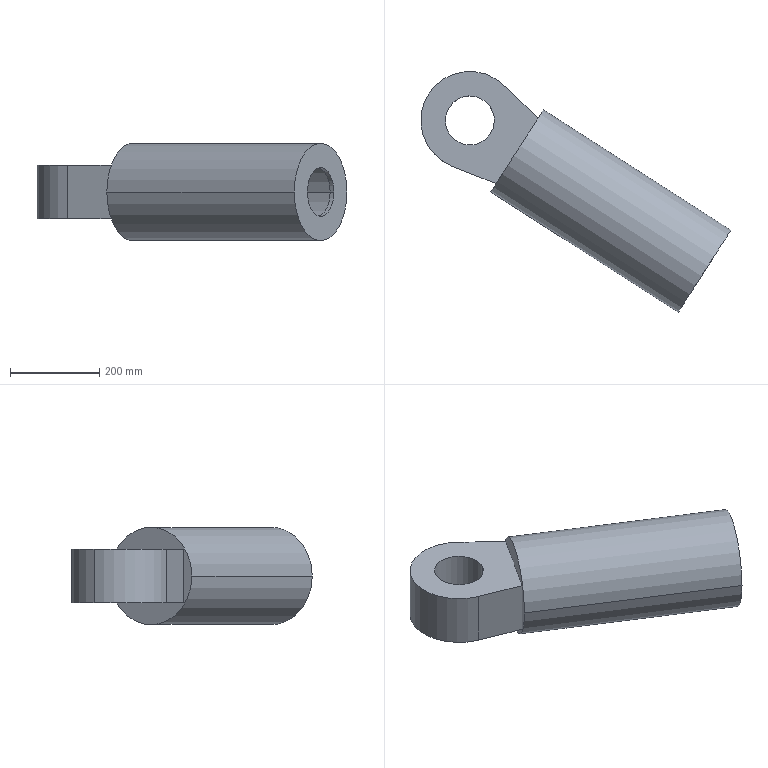Part | SolidWorks | features SplitBody 1 | 1 solid | 18 faces | box 696.192 x 540.383 x 219 mm | volume 10939320 mm3 | cylinder 10 | plane 8 | commonest cylinder face diameters 110 x4 180 x2 219 x2 220 x2
STEP:
#1=CARTESIAN_POINT('',(4022.192,522.369,927.5));
#2=VERTEX_POINT('',#1);
#3=CARTESIAN_POINT('',(3903.913,338.057,927.5));
#4=VERTEX_POINT('',#3);
#5=CARTESIAN_POINT('',(3963.053,430.213,927.5));
#6=DIRECTION('',(-0.8416,0.5401,0.));
#7=DIRECTION('',(0.5401,0.8416,0.));
#8=AXIS2_PLACEMENT_3D('',#5,#6,#7);
#9=CIRCLE('',#8,109.5);
#10=EDGE_CURVE('',#2,#4,#9,.T.);
#11=ORIENTED_EDGE('',*,*,#10,.T.);
#12=CARTESIAN_POINT('',(3483.109,608.101,927.5));
#13=VERTEX_POINT('',#12);
#14=CARTESIAN_POINT('',(3903.913,338.057,927.5));
#15=DIRECTION('',(-0.8416,0.5401,0.));
#16=VECTOR('',#15,1000.);
#17=LINE('',#14,#16);
#18=EDGE_CURVE('',#4,#13,#17,.T.);
#19=ORIENTED_EDGE('',*,*,#18,.T.);
#20=CARTESIAN_POINT('',(3601.388,792.413,927.5));
#21=VERTEX_POINT('',#20);
#22=CARTESIAN_POINT('',(3542.248,700.257,927.5));
#23=DIRECTION('',(0.8416,-0.5401,0.));
#24=DIRECTION('',(0.5401,0.8416,0.));
#25=AXIS2_PLACEMENT_3D('',#22,#23,#24);
#26=CIRCLE('',#25,109.5);
#27=EDGE_CURVE('',#13,#21,#26,.T.);
#28=ORIENTED_EDGE('',*,*,#27,.T.);
#29=CARTESIAN_POINT('',(4022.192,522.369,927.5));
#30=DIRECTION('',(-0.8416,0.5401,0.));
#31=VECTOR('',#30,1000.);
#32=LINE('',#29,#31);
#33=EDGE_CURVE('',#2,#21,#32,.T.);
#34=ORIENTED_EDGE('',*,*,#33,.F.);
#35=EDGE_LOOP('',(#11,#19,#28,#34));
#36=FACE_OUTER_BOUND('',#35,.T.);
#37=CARTESIAN_POINT('',(3963.053,430.213,927.5));
#38=DIRECTION('',(-0.8416,0.5401,0.));
#39=DIRECTION('',(0.5401,0.8416,0.));
#40=AXIS2_PLACEMENT_3D('',#37,#38,#39);
#41=CYLINDRICAL_SURFACE('',#40,109.5);
#42=ADVANCED_FACE('',(#36),#41,.T.);
#43=CARTESIAN_POINT('',(3984.341,481.902,927.5));
#44=VERTEX_POINT('',#43);
#45=CARTESIAN_POINT('',(3924.932,389.325,927.5));
#46=VERTEX_POINT('',#45);
#47=CARTESIAN_POINT('',(3954.637,435.614,927.5));
#48=DIRECTION('',(0.8416,-0.5401,0.));
#49=DIRECTION('',(-0.5401,-0.8416,0.));
#50=AXIS2_PLACEMENT_3D('',#47,#48,#49);
#51=CIRCLE('',#50,55.);
#52=EDGE_CURVE('',#44,#46,#51,.T.);
#53=ORIENTED_EDGE('',*,*,#52,.F.);
#54=CARTESIAN_POINT('',(3992.757,476.501,927.5));
#55=VERTEX_POINT('',#54);
#56=CARTESIAN_POINT('',(3984.341,481.902,927.5));
#57=DIRECTION('',(0.8416,-0.5401,0.));
#58=VECTOR('',#57,1000.);
#59=LINE('',#56,#58);
#60=EDGE_CURVE('',#44,#55,#59,.T.);
#61=ORIENTED_EDGE('',*,*,#60,.T.);
#62=CARTESIAN_POINT('',(3933.348,383.924,927.5));
#63=VERTEX_POINT('',#62);
#64=CARTESIAN_POINT('',(3963.053,430.213,927.5));
#65=DIRECTION('',(-0.8416,0.5401,0.));
#66=DIRECTION('',(-0.5401,-0.8416,0.));
#67=AXIS2_PLACEMENT_3D('',#64,#65,#66);
#68=CIRCLE('',#67,55.);
#69=EDGE_CURVE('',#63,#55,#68,.T.);
#70=ORIENTED_EDGE('',*,*,#69,.F.);
#71=CARTESIAN_POINT('',(3924.932,389.325,927.5));
#72=DIRECTION('',(0.8416,-0.5401,0.));
#73=VECTOR('',#72,1000.);
#74=LINE('',#71,#73);
#75=EDGE_CURVE('',#46,#63,#74,.T.);
#76=ORIENTED_EDGE('',*,*,#75,.F.);
#77=EDGE_LOOP('',(#53,#61,#70,#76));
#78=FACE_OUTER_BOUND('',#77,.T.);
#79=CARTESIAN_POINT('',(3954.637,435.614,927.5));
#80=DIRECTION('',(0.8416,-0.5401,0.));
#81=DIRECTION('',(-0.5401,-0.8416,0.));
#82=AXIS2_PLACEMENT_3D('',#79,#80,#81);
#83=CYLINDRICAL_SURFACE('',#82,55.);
#84=ADVANCED_FACE('',(#78),#83,.F.);
#85=CARTESIAN_POINT('',(3343.423,827.85,867.5));
#86=VERTEX_POINT('',#85);
#87=CARTESIAN_POINT('',(3511.997,847.967,867.5));
#88=VERTEX_POINT('',#87);
#89=CARTESIAN_POINT('',(3436.,768.44,867.5));
#90=DIRECTION('',(0.,0.,-1.));
#91=DIRECTION('',(-0.8416,0.5401,0.));
#92=AXIS2_PLACEMENT_3D('',#89,#90,#91);
#93=CIRCLE('',#92,110.);
#94=EDGE_CURVE('',#86,#88,#93,.T.);
#95=ORIENTED_EDGE('',*,*,#94,.F.);
#96=CARTESIAN_POINT('',(3343.423,827.85,987.5));
#97=VERTEX_POINT('',#96);
#98=CARTESIAN_POINT('',(3343.423,827.85,867.5));
#99=DIRECTION('',(0.,0.,1.));
#100=VECTOR('',#99,1000.);
#101=LINE('',#98,#100);
#102=EDGE_CURVE('',#86,#97,#101,.T.);
#103=ORIENTED_EDGE('',*,*,#102,.T.);
#104=CARTESIAN_POINT('',(3511.997,847.967,987.5));
#105=VERTEX_POINT('',#104);
#106=CARTESIAN_POINT('',(3436.,768.44,987.5));
#107=DIRECTION('',(0.,0.,-1.));
#108=DIRECTION('',(-0.8416,0.5401,0.));
#109=AXIS2_PLACEMENT_3D('',#106,#107,#108);
#110=CIRCLE('',#109,110.);
#111=EDGE_CURVE('',#97,#105,#110,.T.);
#112=ORIENTED_EDGE('',*,*,#111,.T.);
#113=CARTESIAN_POINT('',(3511.997,847.967,867.5));
#114=DIRECTION('',(0.,0.,-1.));
#115=VECTOR('',#114,1000.);
#116=LINE('',#113,#115);
#117=EDGE_CURVE('',#105,#88,#116,.T.);
#118=ORIENTED_EDGE('',*,*,#117,.T.);
#119=EDGE_LOOP('',(#95,#103,#112,#118));
#120=FACE_OUTER_BOUND('',#119,.T.);
#121=CARTESIAN_POINT('',(3436.,768.44,867.5));
#122=DIRECTION('',(0.,0.,1.));
#123=DIRECTION('',(-0.8416,0.5401,0.));
#124=AXIS2_PLACEMENT_3D('',#121,#122,#123);
#125=CYLINDRICAL_SURFACE('',#124,110.);
#126=ADVANCED_FACE('',(#120),#125,.T.);
#127=CARTESIAN_POINT('',(3482.288,738.735,867.5));
#128=VERTEX_POINT('',#127);
#129=CARTESIAN_POINT('',(3389.712,798.145,867.5));
#130=VERTEX_POINT('',#129);
#131=CARTESIAN_POINT('',(3436.,768.44,867.5));
#132=DIRECTION('',(0.,0.,1.));
#133=DIRECTION('',(-0.8416,0.5401,0.));
#134=AXIS2_PLACEMENT_3D('',#131,#132,#133);
#135=CIRCLE('',#134,55.);
#136=EDGE_CURVE('',#128,#130,#135,.T.);
#137=ORIENTED_EDGE('',*,*,#136,.F.);
#138=CARTESIAN_POINT('',(3482.288,738.735,987.5));
#139=VERTEX_POINT('',#138);
#140=CARTESIAN_POINT('',(3482.288,738.735,867.5));
#141=DIRECTION('',(0.,0.,1.));
#142=VECTOR('',#141,1000.);
#143=LINE('',#140,#142);
#144=EDGE_CURVE('',#128,#139,#143,.T.);
#145=ORIENTED_EDGE('',*,*,#144,.T.);
#146=CARTESIAN_POINT('',(3389.712,798.145,987.5));
#147=VERTEX_POINT('',#146);
#148=CARTESIAN_POINT('',(3436.,768.44,987.5));
#149=DIRECTION('',(0.,0.,1.));
#150=DIRECTION('',(-0.8416,0.5401,0.));
#151=AXIS2_PLACEMENT_3D('',#148,#149,#150);
#152=CIRCLE('',#151,55.);
#153=EDGE_CURVE('',#139,#147,#152,.T.);
#154=ORIENTED_EDGE('',*,*,#153,.T.);
#155=CARTESIAN_POINT('',(3389.712,798.145,867.5));
#156=DIRECTION('',(0.,0.,1.));
#157=VECTOR('',#156,1000.);
#158=LINE('',#155,#157);
#159=EDGE_CURVE('',#130,#147,#158,.T.);
#160=ORIENTED_EDGE('',*,*,#159,.F.);
#161=EDGE_LOOP('',(#137,#145,#154,#160));
#162=FACE_OUTER_BOUND('',#161,.T.);
#163=CARTESIAN_POINT('',(3436.,768.44,867.5));
#164=DIRECTION('',(0.,0.,1.));
#165=DIRECTION('',(-0.8416,0.5401,0.));
#166=AXIS2_PLACEMENT_3D('',#163,#164,#165);
#167=CYLINDRICAL_SURFACE('',#166,55.);
#168=ADVANCED_FACE('',(#162),#167,.F.);
#169=CARTESIAN_POINT('',(3607.689,765.2,927.5));
#170=VERTEX_POINT('',#169);
#171=CARTESIAN_POINT('',(3510.473,613.71,927.5));
#172=VERTEX_POINT('',#171);
#173=CARTESIAN_POINT('',(3559.081,689.455,927.5));
#174=DIRECTION('',(0.8416,-0.5401,0.));
#175=DIRECTION('',(-0.5401,-0.8416,0.));
#176=AXIS2_PLACEMENT_3D('',#173,#174,#175);
#177=CIRCLE('',#176,90.);
#178=EDGE_CURVE('',#170,#172,#177,.T.);
#179=ORIENTED_EDGE('',*,*,#178,.F.);
#180=CARTESIAN_POINT('',(4003.244,511.358,927.5));
#181=VERTEX_POINT('',#180);
#182=CARTESIAN_POINT('',(3607.689,765.2,927.5));
#183=DIRECTION('',(0.8416,-0.5401,0.));
#184=VECTOR('',#183,1000.);
#185=LINE('',#182,#184);
#186=EDGE_CURVE('',#170,#181,#185,.T.);
#187=ORIENTED_EDGE('',*,*,#186,.T.);
#188=CARTESIAN_POINT('',(3906.029,359.869,927.5));
#189=VERTEX_POINT('',#188);
#190=CARTESIAN_POINT('',(3954.637,435.614,927.5));
#191=DIRECTION('',(0.8416,-0.5401,0.));
#192=DIRECTION('',(-0.5401,-0.8416,0.));
#193=AXIS2_PLACEMENT_3D('',#190,#191,#192);
#194=CIRCLE('',#193,90.);
#195=EDGE_CURVE('',#181,#189,#194,.T.);
#196=ORIENTED_EDGE('',*,*,#195,.T.);
#197=CARTESIAN_POINT('',(3510.473,613.71,927.5));
#198=DIRECTION('',(0.8416,-0.5401,0.));
#199=VECTOR('',#198,1000.);
#200=LINE('',#197,#199);
#201=EDGE_CURVE('',#172,#189,#200,.T.);
#202=ORIENTED_EDGE('',*,*,#201,.F.);
#203=EDGE_LOOP('',(#179,#187,#196,#202));
#204=FACE_OUTER_BOUND('',#203,.T.);
#205=CARTESIAN_POINT('',(3559.081,689.455,927.5));
#206=DIRECTION('',(0.8416,-0.5401,0.));
#207=DIRECTION('',(-0.5401,-0.8416,0.));
#208=AXIS2_PLACEMENT_3D('',#205,#206,#207);
#209=CYLINDRICAL_SURFACE('',#208,90.);
#210=ADVANCED_FACE('',(#204),#209,.F.);
#211=ORIENTED_EDGE('',*,*,#18,.F.);
#212=CARTESIAN_POINT('',(3963.053,430.213,927.5));
#213=DIRECTION('',(-0.8416,0.5401,0.));
#214=DIRECTION('',(0.5401,0.8416,0.));
#215=AXIS2_PLACEMENT_3D('',#212,#213,#214);
#216=CIRCLE('',#215,109.5);
#217=EDGE_CURVE('',#4,#2,#216,.T.);
#218=ORIENTED_EDGE('',*,*,#217,.T.);
#219=ORIENTED_EDGE('',*,*,#33,.T.);
#220=CARTESIAN_POINT('',(3542.248,700.257,927.5));
#221=DIRECTION('',(0.8416,-0.5401,0.));
#222=DIRECTION('',(0.5401,0.8416,0.));
#223=AXIS2_PLACEMENT_3D('',#220,#221,#222);
#224=CIRCLE('',#223,109.5);
#225=EDGE_CURVE('',#21,#13,#224,.T.);
#226=ORIENTED_EDGE('',*,*,#225,.T.);
#227=EDGE_LOOP('',(#211,#218,#219,#226));
#228=FACE_OUTER_BOUND('',#227,.T.);
#229=CARTESIAN_POINT('',(3963.053,430.213,927.5));
#230=DIRECTION('',(-0.8416,0.5401,0.));
#231=DIRECTION('',(0.5401,0.8416,0.));
#232=AXIS2_PLACEMENT_3D('',#229,#230,#231);
#233=CYLINDRICAL_SURFACE('',#232,109.5);
#234=ADVANCED_FACE('',(#228),#233,.T.);
#235=CARTESIAN_POINT('',(3494.991,626.616,987.5));
#236=VERTEX_POINT('',#235);
#237=CARTESIAN_POINT('',(3589.506,773.898,987.5));
#238=VERTEX_POINT('',#237);
#239=CARTESIAN_POINT('',(3542.248,700.257,987.5));
#240=DIRECTION('',(0.5401,0.8416,0.));
#241=VECTOR('',#240,1000.);
#242=LINE('',#239,#241);
#243=EDGE_CURVE('',#236,#238,#242,.T.);
#244=ORIENTED_EDGE('',*,*,#243,.F.);
#245=CARTESIAN_POINT('',(3494.991,626.616,867.5));
#246=VERTEX_POINT('',#245);
#247=CARTESIAN_POINT('',(3494.991,626.616,927.5));
#248=DIRECTION('',(0.,0.,1.));
#249=VECTOR('',#248,1000.);
#250=LINE('',#247,#249);
#251=EDGE_CURVE('',#246,#236,#250,.T.);
#252=ORIENTED_EDGE('',*,*,#251,.F.);
#253=CARTESIAN_POINT('',(3589.506,773.898,867.5));
#254=VERTEX_POINT('',#253);
#255=CARTESIAN_POINT('',(3542.248,700.257,867.5));
#256=DIRECTION('',(-0.5401,-0.8416,0.));
#257=VECTOR('',#256,1000.);
#258=LINE('',#255,#257);
#259=EDGE_CURVE('',#254,#246,#258,.T.);
#260=ORIENTED_EDGE('',*,*,#259,.F.);
#261=CARTESIAN_POINT('',(3589.506,773.898,927.5));
#262=DIRECTION('',(0.,0.,-1.));
#263=VECTOR('',#262,1000.);
#264=LINE('',#261,#263);
#265=EDGE_CURVE('',#238,#254,#264,.T.);
#266=ORIENTED_EDGE('',*,*,#265,.F.);
#267=EDGE_LOOP('',(#244,#252,#260,#266));
#268=FACE_BOUND('',#267,.T.);
#269=ORIENTED_EDGE('',*,*,#225,.F.);
#270=ORIENTED_EDGE('',*,*,#27,.F.);
#271=EDGE_LOOP('',(#269,#270));
#272=FACE_OUTER_BOUND('',#271,.T.);
#273=CARTESIAN_POINT('',(3542.248,700.257,927.5));
#274=DIRECTION('',(0.8416,-0.5401,0.));
#275=DIRECTION('',(-0.5401,-0.8416,0.));
#276=AXIS2_PLACEMENT_3D('',#273,#274,#275);
#277=PLANE('',#276);
#278=ADVANCED_FACE('',(#268,#272),#277,.F.);
#279=ORIENTED_EDGE('',*,*,#69,.T.);
#280=CARTESIAN_POINT('',(3963.053,430.213,927.5));
#281=DIRECTION('',(-0.8416,0.5401,0.));
#282=DIRECTION('',(-0.5401,-0.8416,0.));
#283=AXIS2_PLACEMENT_3D('',#280,#281,#282);
#284=CIRCLE('',#283,55.);
#285=EDGE_CURVE('',#55,#63,#284,.T.);
#286=ORIENTED_EDGE('',*,*,#285,.T.);
#287=EDGE_LOOP('',(#279,#286));
#288=FACE_BOUND('',#287,.T.);
#289=ORIENTED_EDGE('',*,*,#10,.F.);
#290=ORIENTED_EDGE('',*,*,#217,.F.);
#291=EDGE_LOOP('',(#289,#290));
#292=FACE_OUTER_BOUND('',#291,.T.);
#293=CARTESIAN_POINT('',(3963.053,430.213,927.5));
#294=DIRECTION('',(0.8416,-0.5401,0.));
#295=DIRECTION('',(-0.5401,-0.8416,0.));
#296=AXIS2_PLACEMENT_3D('',#293,#294,#295);
#297=PLANE('',#296);
#298=ADVANCED_FACE('',(#288,#292),#297,.T.);
#299=ORIENTED_EDGE('',*,*,#265,.T.);
#300=CARTESIAN_POINT('',(3511.997,847.967,867.5));
#301=DIRECTION('',(0.723,-0.6909,0.));
#302=VECTOR('',#301,1000.);
#303=LINE('',#300,#302);
#304=EDGE_CURVE('',#88,#254,#303,.T.);
#305=ORIENTED_EDGE('',*,*,#304,.F.);
#306=ORIENTED_EDGE('',*,*,#117,.F.);
#307=CARTESIAN_POINT('',(3511.997,847.967,987.5));
#308=DIRECTION('',(-0.723,0.6909,0.));
#309=VECTOR('',#308,1000.);
#310=LINE('',#307,#309);
#311=EDGE_CURVE('',#238,#105,#310,.T.);
#312=ORIENTED_EDGE('',*,*,#311,.F.);
#313=EDGE_LOOP('',(#299,#305,#306,#312));
#314=FACE_OUTER_BOUND('',#313,.T.);
#315=CARTESIAN_POINT('',(3511.997,847.967,867.5));
#316=DIRECTION('',(-0.6909,-0.723,0.));
#317=DIRECTION('',(-0.723,0.6909,0.));
#318=AXIS2_PLACEMENT_3D('',#315,#316,#317);
#319=PLANE('',#318);
#320=ADVANCED_FACE('',(#314),#319,.F.);
#321=CARTESIAN_POINT('',(3436.,768.44,987.5));
#322=DIRECTION('',(0.,0.,1.));
#323=DIRECTION('',(-0.8416,0.5401,0.));
#324=AXIS2_PLACEMENT_3D('',#321,#322,#323);
#325=CIRCLE('',#324,55.);
#326=EDGE_CURVE('',#147,#139,#325,.T.);
#327=ORIENTED_EDGE('',*,*,#326,.F.);
#328=ORIENTED_EDGE('',*,*,#153,.F.);
#329=EDGE_LOOP('',(#327,#328));
#330=FACE_BOUND('',#329,.T.);
#331=CARTESIAN_POINT('',(3395.364,666.221,987.5));
#332=VERTEX_POINT('',#331);
#333=CARTESIAN_POINT('',(3494.991,626.616,987.5));
#334=DIRECTION('',(-0.9293,0.3694,0.));
#335=VECTOR('',#334,1000.);
#336=LINE('',#333,#335);
#337=EDGE_CURVE('',#236,#332,#336,.T.);
#338=ORIENTED_EDGE('',*,*,#337,.F.);
#339=ORIENTED_EDGE('',*,*,#243,.T.);
#340=ORIENTED_EDGE('',*,*,#311,.T.);
#341=ORIENTED_EDGE('',*,*,#111,.F.);
#342=CARTESIAN_POINT('',(3436.,768.44,987.5));
#343=DIRECTION('',(0.,0.,-1.));
#344=DIRECTION('',(-0.8416,0.5401,0.));
#345=AXIS2_PLACEMENT_3D('',#342,#343,#344);
#346=CIRCLE('',#345,110.);
#347=EDGE_CURVE('',#332,#97,#346,.T.);
#348=ORIENTED_EDGE('',*,*,#347,.F.);
#349=EDGE_LOOP('',(#338,#339,#340,#341,#348));
#350=FACE_OUTER_BOUND('',#349,.T.);
#351=CARTESIAN_POINT('',(3436.,768.44,987.5));
#352=DIRECTION('',(0.,0.,-1.));
#353=DIRECTION('',(0.8416,-0.5401,0.));
#354=AXIS2_PLACEMENT_3D('',#351,#352,#353);
#355=PLANE('',#354);
#356=ADVANCED_FACE('',(#330,#350),#355,.F.);
#357=CARTESIAN_POINT('',(3395.364,666.221,867.5));
#358=VERTEX_POINT('',#357);
#359=CARTESIAN_POINT('',(3395.364,666.221,867.5));
#360=DIRECTION('',(0.,0.,1.));
#361=VECTOR('',#360,1000.);
#362=LINE('',#359,#361);
#363=EDGE_CURVE('',#358,#332,#362,.T.);
#364=ORIENTED_EDGE('',*,*,#363,.F.);
#365=CARTESIAN_POINT('',(3395.364,666.221,867.5));
#366=DIRECTION('',(-0.9293,0.3694,0.));
#367=VECTOR('',#366,1000.);
#368=LINE('',#365,#367);
#369=EDGE_CURVE('',#246,#358,#368,.T.);
#370=ORIENTED_EDGE('',*,*,#369,.F.);
#371=ORIENTED_EDGE('',*,*,#251,.T.);
#372=ORIENTED_EDGE('',*,*,#337,.T.);
#373=EDGE_LOOP('',(#364,#370,#371,#372));
#374=FACE_OUTER_BOUND('',#373,.T.);
#375=CARTESIAN_POINT('',(3395.364,666.221,867.5));
#376=DIRECTION('',(0.3694,0.9293,0.));
#377=DIRECTION('',(0.9293,-0.3694,0.));
#378=AXIS2_PLACEMENT_3D('',#375,#376,#377);
#379=PLANE('',#378);
#380=ADVANCED_FACE('',(#374),#379,.F.);
#381=CARTESIAN_POINT('',(3436.,768.44,867.5));
#382=DIRECTION('',(0.,0.,1.));
#383=DIRECTION('',(-0.8416,0.5401,0.));
#384=AXIS2_PLACEMENT_3D('',#381,#382,#383);
#385=CIRCLE('',#384,55.);
#386=EDGE_CURVE('',#130,#128,#385,.T.);
#387=ORIENTED_EDGE('',*,*,#386,.T.);
#388=ORIENTED_EDGE('',*,*,#136,.T.);
#389=EDGE_LOOP('',(#387,#388));
#390=FACE_BOUND('',#389,.T.);
#391=ORIENTED_EDGE('',*,*,#259,.T.);
#392=ORIENTED_EDGE('',*,*,#369,.T.);
#393=CARTESIAN_POINT('',(3436.,768.44,867.5));
#394=DIRECTION('',(0.,0.,-1.));
#395=DIRECTION('',(-0.8416,0.5401,0.));
#396=AXIS2_PLACEMENT_3D('',#393,#394,#395);
#397=CIRCLE('',#396,110.);
#398=EDGE_CURVE('',#358,#86,#397,.T.);
#399=ORIENTED_EDGE('',*,*,#398,.T.);
#400=ORIENTED_EDGE('',*,*,#94,.T.);
#401=ORIENTED_EDGE('',*,*,#304,.T.);
#402=EDGE_LOOP('',(#391,#392,#399,#400,#401));
#403=FACE_OUTER_BOUND('',#402,.T.);
#404=CARTESIAN_POINT('',(3436.,768.44,867.5));
#405=DIRECTION('',(0.,0.,-1.));
#406=DIRECTION('',(0.8416,-0.5401,0.));
#407=AXIS2_PLACEMENT_3D('',#404,#405,#406);
#408=PLANE('',#407);
#409=ADVANCED_FACE('',(#390,#403),#408,.T.);
#410=ORIENTED_EDGE('',*,*,#60,.F.);
#411=CARTESIAN_POINT('',(3954.637,435.614,927.5));
#412=DIRECTION('',(0.8416,-0.5401,0.));
#413=DIRECTION('',(-0.5401,-0.8416,0.));
#414=AXIS2_PLACEMENT_3D('',#411,#412,#413);
#415=CIRCLE('',#414,55.);
#416=EDGE_CURVE('',#46,#44,#415,.T.);
#417=ORIENTED_EDGE('',*,*,#416,.F.);
#418=ORIENTED_EDGE('',*,*,#75,.T.);
#419=ORIENTED_EDGE('',*,*,#285,.F.);
#420=EDGE_LOOP('',(#410,#417,#418,#419));
#421=FACE_OUTER_BOUND('',#420,.T.);
#422=CARTESIAN_POINT('',(3954.637,435.614,927.5));
#423=DIRECTION('',(0.8416,-0.5401,0.));
#424=DIRECTION('',(-0.5401,-0.8416,0.));
#425=AXIS2_PLACEMENT_3D('',#422,#423,#424);
#426=CYLINDRICAL_SURFACE('',#425,55.);
#427=ADVANCED_FACE('',(#421),#426,.F.);
#428=ORIENTED_EDGE('',*,*,#102,.F.);
#429=ORIENTED_EDGE('',*,*,#398,.F.);
#430=ORIENTED_EDGE('',*,*,#363,.T.);
#431=ORIENTED_EDGE('',*,*,#347,.T.);
#432=EDGE_LOOP('',(#428,#429,#430,#431));
#433=FACE_OUTER_BOUND('',#432,.T.);
#434=CARTESIAN_POINT('',(3436.,768.44,867.5));
#435=DIRECTION('',(0.,0.,1.));
#436=DIRECTION('',(-0.8416,0.5401,0.));
#437=AXIS2_PLACEMENT_3D('',#434,#435,#436);
#438=CYLINDRICAL_SURFACE('',#437,110.);
#439=ADVANCED_FACE('',(#433),#438,.T.);
#440=ORIENTED_EDGE('',*,*,#144,.F.);
#441=ORIENTED_EDGE('',*,*,#386,.F.);
#442=ORIENTED_EDGE('',*,*,#159,.T.);
#443=ORIENTED_EDGE('',*,*,#326,.T.);
#444=EDGE_LOOP('',(#440,#441,#442,#443));
#445=FACE_OUTER_BOUND('',#444,.T.);
#446=CARTESIAN_POINT('',(3436.,768.44,867.5));
#447=DIRECTION('',(0.,0.,1.));
#448=DIRECTION('',(-0.8416,0.5401,0.));
#449=AXIS2_PLACEMENT_3D('',#446,#447,#448);
#450=CYLINDRICAL_SURFACE('',#449,55.);
#451=ADVANCED_FACE('',(#445),#450,.F.);
#452=CARTESIAN_POINT('',(3954.637,435.614,927.5));
#453=DIRECTION('',(0.8416,-0.5401,0.));
#454=DIRECTION('',(-0.5401,-0.8416,0.));
#455=AXIS2_PLACEMENT_3D('',#452,#453,#454);
#456=CIRCLE('',#455,90.);
#457=EDGE_CURVE('',#189,#181,#456,.T.);
#458=ORIENTED_EDGE('',*,*,#457,.F.);
#459=ORIENTED_EDGE('',*,*,#195,.F.);
#460=EDGE_LOOP('',(#458,#459));
#461=FACE_OUTER_BOUND('',#460,.T.);
#462=ORIENTED_EDGE('',*,*,#416,.T.);
#463=ORIENTED_EDGE('',*,*,#52,.T.);
#464=EDGE_LOOP('',(#462,#463));
#465=FACE_BOUND('',#464,.T.);
#466=CARTESIAN_POINT('',(3954.637,435.614,927.5));
#467=DIRECTION('',(0.8416,-0.5401,0.));
#468=DIRECTION('',(-0.5401,-0.8416,0.));
#469=AXIS2_PLACEMENT_3D('',#466,#467,#468);
#470=PLANE('',#469);
#471=ADVANCED_FACE('',(#461,#465),#470,.F.);
#472=ORIENTED_EDGE('',*,*,#186,.F.);
#473=CARTESIAN_POINT('',(3559.081,689.455,927.5));
#474=DIRECTION('',(0.8416,-0.5401,0.));
#475=DIRECTION('',(-0.5401,-0.8416,0.));
#476=AXIS2_PLACEMENT_3D('',#473,#474,#475);
#477=CIRCLE('',#476,90.);
#478=EDGE_CURVE('',#172,#170,#477,.T.);
#479=ORIENTED_EDGE('',*,*,#478,.F.);
#480=ORIENTED_EDGE('',*,*,#201,.T.);
#481=ORIENTED_EDGE('',*,*,#457,.T.);
#482=EDGE_LOOP('',(#472,#479,#480,#481));
#483=FACE_OUTER_BOUND('',#482,.T.);
#484=CARTESIAN_POINT('',(3559.081,689.455,927.5));
#485=DIRECTION('',(0.8416,-0.5401,0.));
#486=DIRECTION('',(-0.5401,-0.8416,0.));
#487=AXIS2_PLACEMENT_3D('',#484,#485,#486);
#488=CYLINDRICAL_SURFACE('',#487,90.);
#489=ADVANCED_FACE('',(#483),#488,.F.);
#490=ORIENTED_EDGE('',*,*,#478,.T.);
#491=ORIENTED_EDGE('',*,*,#178,.T.);
#492=EDGE_LOOP('',(#490,#491));
#493=FACE_OUTER_BOUND('',#492,.T.);
#494=CARTESIAN_POINT('',(3559.081,689.455,927.5));
#495=DIRECTION('',(0.8416,-0.5401,0.));
#496=DIRECTION('',(-0.5401,-0.8416,0.));
#497=AXIS2_PLACEMENT_3D('',#494,#495,#496);
#498=PLANE('',#497);
#499=ADVANCED_FACE('',(#493),#498,.T.);
#500=CLOSED_SHELL('',(#42,#84,#126,#168,#210,#234,#278,#298,#320,#356,#380,#409,#427,#439,#451,#471,#489,#499));
#501=MANIFOLD_SOLID_BREP('',#500);
#502=CARTESIAN_POINT('',(0.,0.,0.));
#503=DIRECTION('',(0.,0.,1.));
#504=DIRECTION('',(1.,0.,0.));
#505=AXIS2_PLACEMENT_3D('',#502,#503,#504);
#506=(LENGTH_UNIT()NAMED_UNIT(*)SI_UNIT(.MILLI.,.METRE.));
#507=UNCERTAINTY_MEASURE_WITH_UNIT(LENGTH_MEASURE(0.00001),#506,'','');
#508=(NAMED_UNIT(*)PLANE_ANGLE_UNIT()SI_UNIT($,.RADIAN.));
#509=(NAMED_UNIT(*)SI_UNIT($,.STERADIAN.)SOLID_ANGLE_UNIT());
#510=(GEOMETRIC_REPRESENTATION_CONTEXT(3)GLOBAL_UNCERTAINTY_ASSIGNED_CONTEXT((#507))GLOBAL_UNIT_ASSIGNED_CONTEXT((#506,#508,#509))REPRESENTATION_CONTEXT('',''));
#511=ADVANCED_BREP_SHAPE_REPRESENTATION('',(#501,#505),#510);